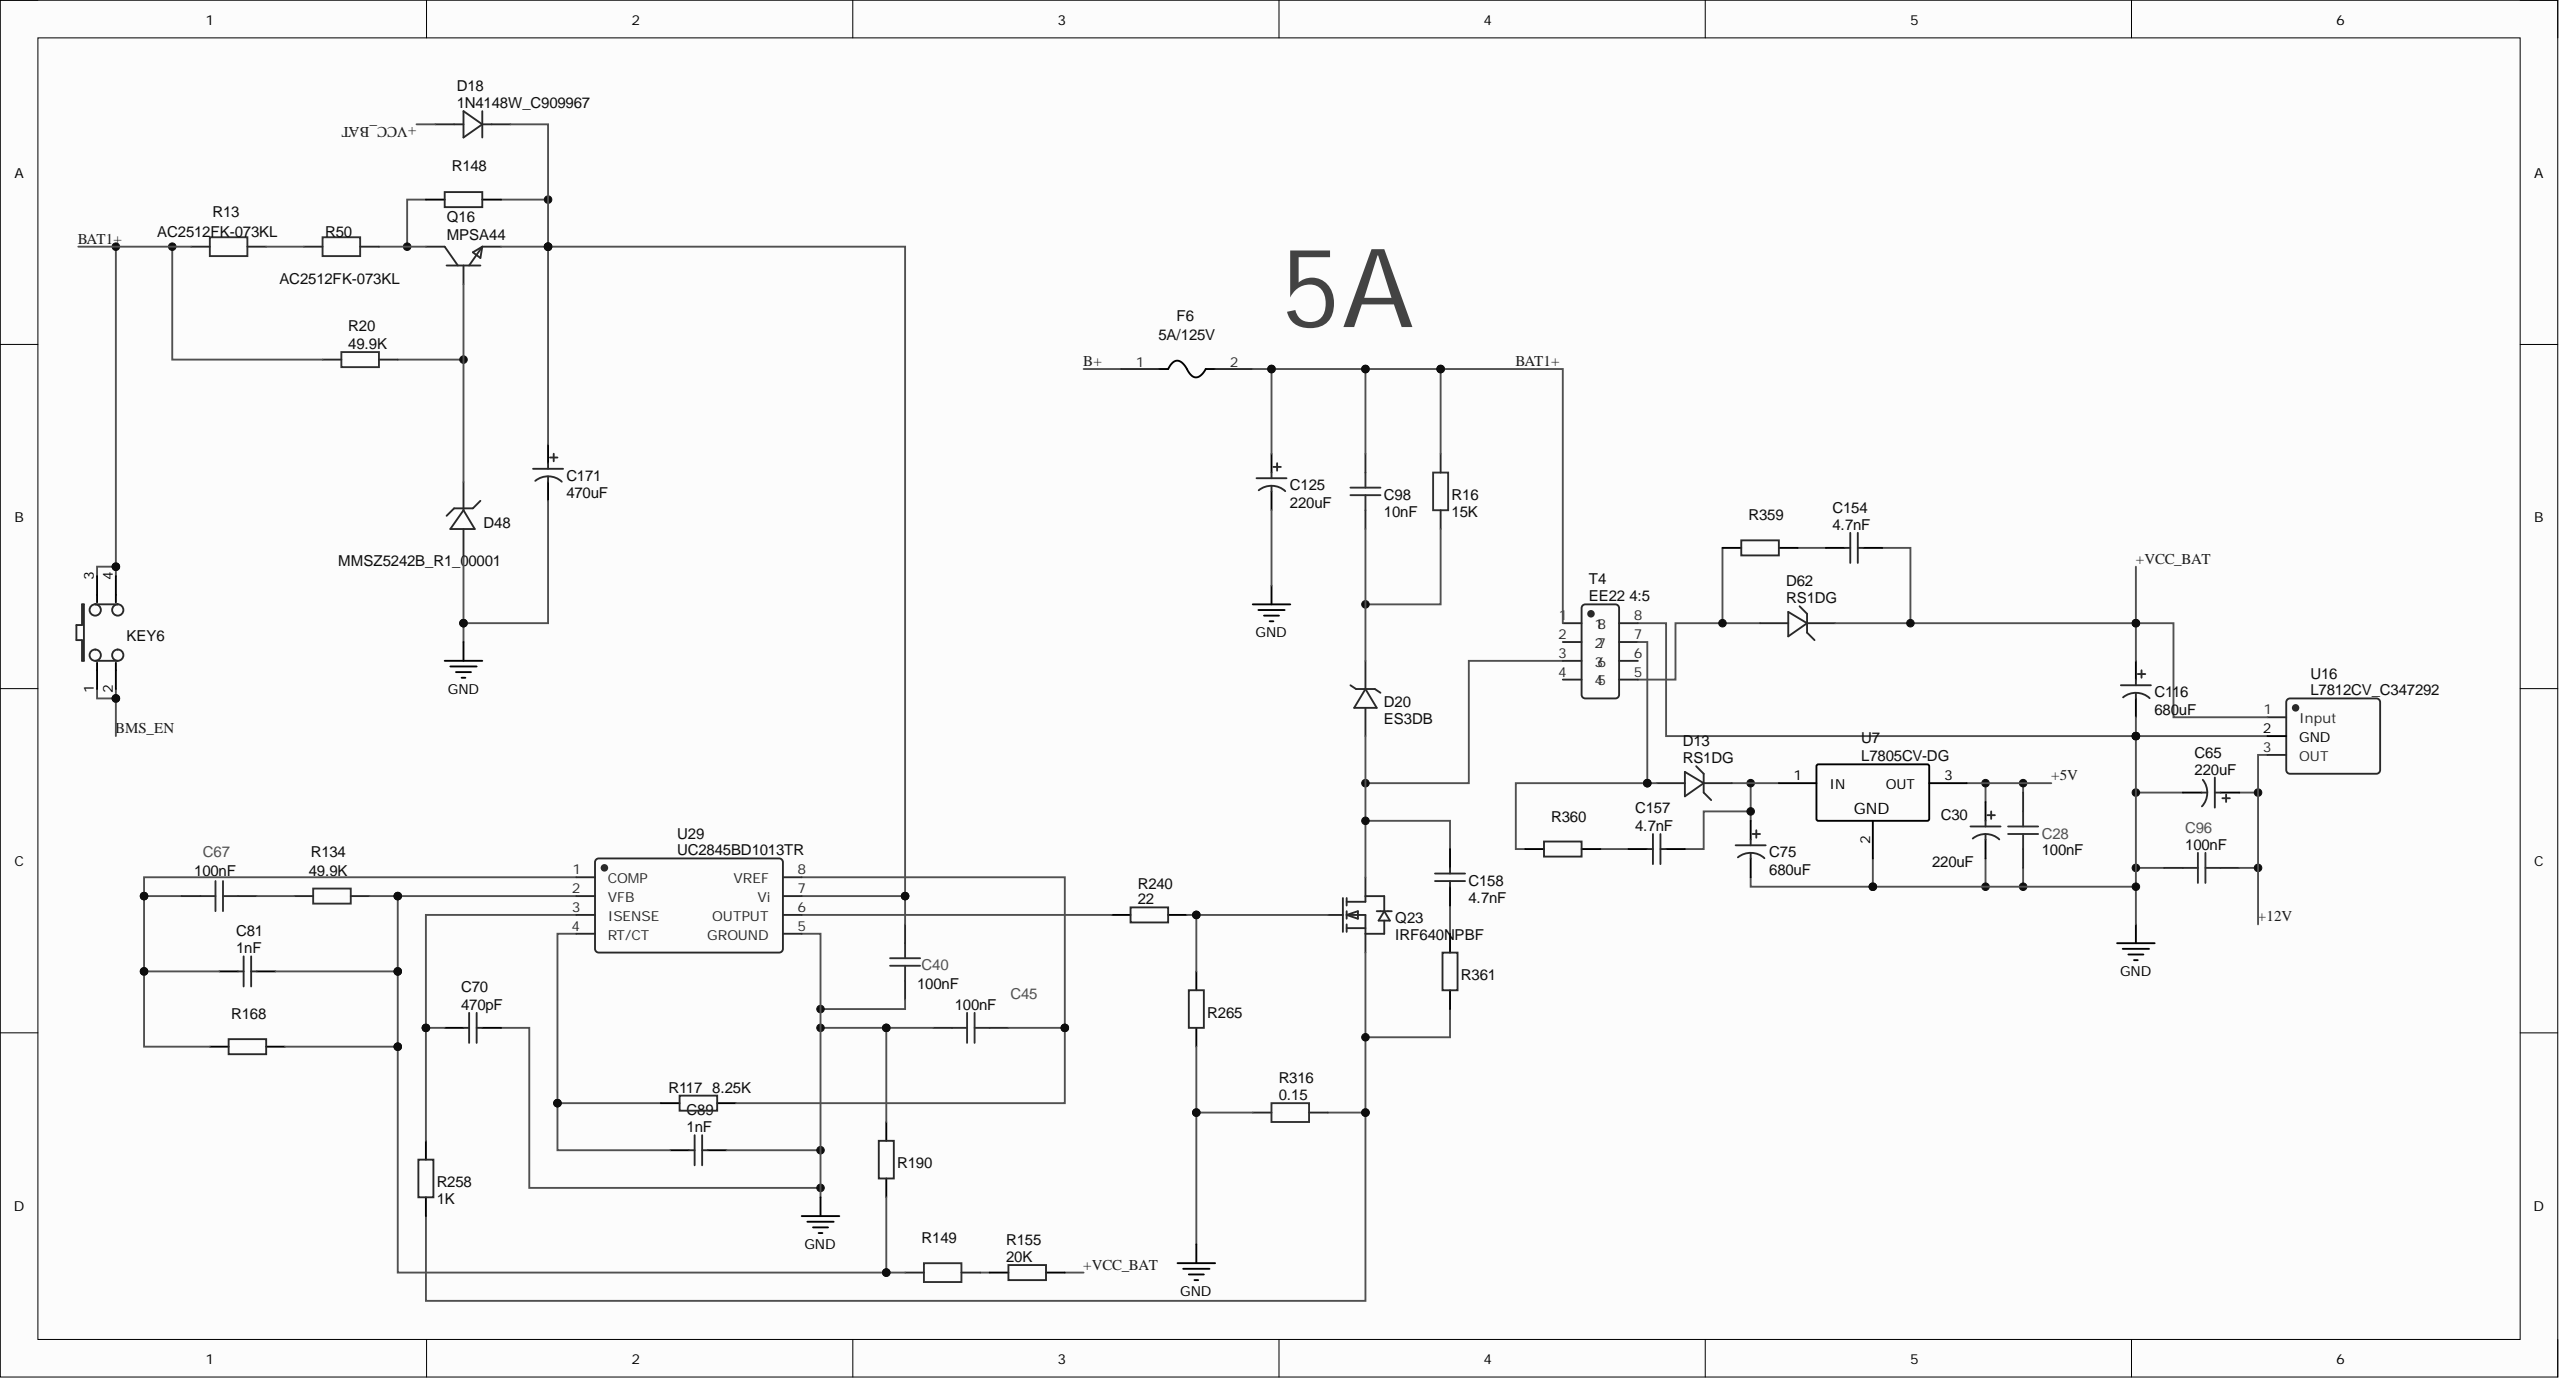Circuit board | Altium Designer | 694 parts | 423 nets | one sheet of the schematic
Parts on this sheet (reference | value | footprint):
C28 | 100nF | C0603
C30 | 220uF | CAP-TH_BD6.3-P2.50-D1.0-FD
C40 | 100nF | C0603
C45 | 100nF | C0603
C65 | 220uF | CAP-TH_BD6.3-P2.50-D1.0-FD
C67 | 100nF | C0603
C70 | 470pF | C0603
C75 | 680uF | CAP-TH_BD10.0-P5.00-D1.0-FD
C81 | 1nF | C0603
C89 | 1nF | C0603
C96 | 100nF | C0603
C98 | 10nF | CAP-TH_L8.0-W4.0-P5.00-D1.2
C116 | 680uF | CAP-TH_BD10.0-P5.00-D1.0-FD
C125 | 220uF | CAP-TH_BD10.0-P5.00-D1.0-FD
C154 | 4.7nF | C1206
C157 | 4.7nF | C1206
C158 | 4.7nF | C1206
C171 | 470uF | CAP-TH_BD12.5-P5.00-D0.6-FD
D13 | RS1DG | SMA_L4.4-W2.8-LS5.4-RD
D18 | 1N4148W_C909967 | SOD-123_L2.8-W1.8-LS3.7-RD
D20 | ES3DB | SMB_L4.6-W3.6-LS5.3-RD
D48 | MMSZ5242B_R1_00001 | SOD-123_L2.7-W1.6-LS3.7-RD-1
D62 | RS1DG | SMA_L4.4-W2.8-LS5.4-RD
F6 | 5A/125V | FUSE-SMD_L6.1-W2.5
KEY6 | 4-1437565-2 | SW-SMD_4P-L6.0-W6.0-P4.50-LS8.6
Q16 | MPSA44 | TO-92-3_L4.8-W3.7-P2.54-L
Q23 | IRF640NPBF | TO-220-3_L10.0-W4.5-P2.54-L
R13 | AC2512FK-073KL | R2512
R16 | 15K | RES-TH_BD3.3-L9.0-P13.00-D0.6
R20 | 49.9K | R0603
R50 | AC2512FK-073KL | R2512
R117 | 8.25K | R0603
R134 | 49.9K | R0603
R148 | R0603
R149 | R0603
R155 | 20K | R0603
R168 | R0603
R190 | R0603
R240 | 22 | R0603
R258 | 1K | R0603
R265 | R0603
R316 | 0.15 | R2512
R359 | R1206
R360 | R1206
R361 | R1206
T4 | EE22 4:5 | EE22 4:5NEW
U7 | L7805CV-DG | TO-220-3_L10.0-W4.5-P2.54-L
U16 | L7812CV_C347292 | TO-220-3_L10.0-W4.5-P2.54-L
U29 | UC2845BD1013TR | SOP-8_L4.9-W3.9-P1.27-LS6.0-BL
Nets of these parts (net: part-pin ...):
NetR240_1: R240-1 U29-6
NetR149_1: R149-1 R155-2
NetR13_1: R13-1 R50-2
NetQ23_3: Q23-3 R258-1 R316-2 R361-1
NetQ23_1: Q23-1 R240-2 R265-2
NetQ16_3: Q16-3 R50-1 R148-1
NetD62_2: D62-2 R359-1 T4-5
NetD48_1: D48-1 Q16-2 R20-2
NetD13_2: D13-2 R360-1 T4-7
NetC158_2: C158-2 D20-2 Q23-2 T4-3
NetC158_1: C158-1 R361-2
NetC157_2: C157-2 R360-2
NetC154_2: C154-2 R359-2
NetC98_1: C98-1 D20-1 R16-1
NetC89_1: C89-1 R117-1 U29-4
NetC81_2: C81-2 R134-2 R149-2 R168-1 R190-1 U29-2
NetC75_1: C75-1 C157-1 D13-1 U7-1
NetC70_1: C70-1 R258-2 U29-3
NetC67_2: C67-2 C81-1 R168-2 U29-1
NetC67_1: C67-1 R134-1
NetC45_1: C45-1 R117-2 U29-8
NetC40_2: C40-2 C171-1 D18-1 Q16-1 R148-2 U29-7
GND: C28-2 C30-2 C40-1 C45-2 C65-2 C70-2 C75-2 C89-2 C96-2 C116-2 C125-2 C171-2 D48-2 R190-2 R265-1 R316-1 T4-8 U7-2 U16-2 U29-5
BMS_EN: KEY6-1 KEY6-2
BAT1+: C98-2 C125-1 F6-2 KEY6-3 KEY6-4 R13-2 R16-2 R20-1 T4-1
B+: F6-1
+VCC_BAT: C116-1 C154-1 D18-2 D62-1 R155-1 U16-1
+12V: C65-1 C96-1 U16-3
+5V: C28-1 C30-1 U7-3